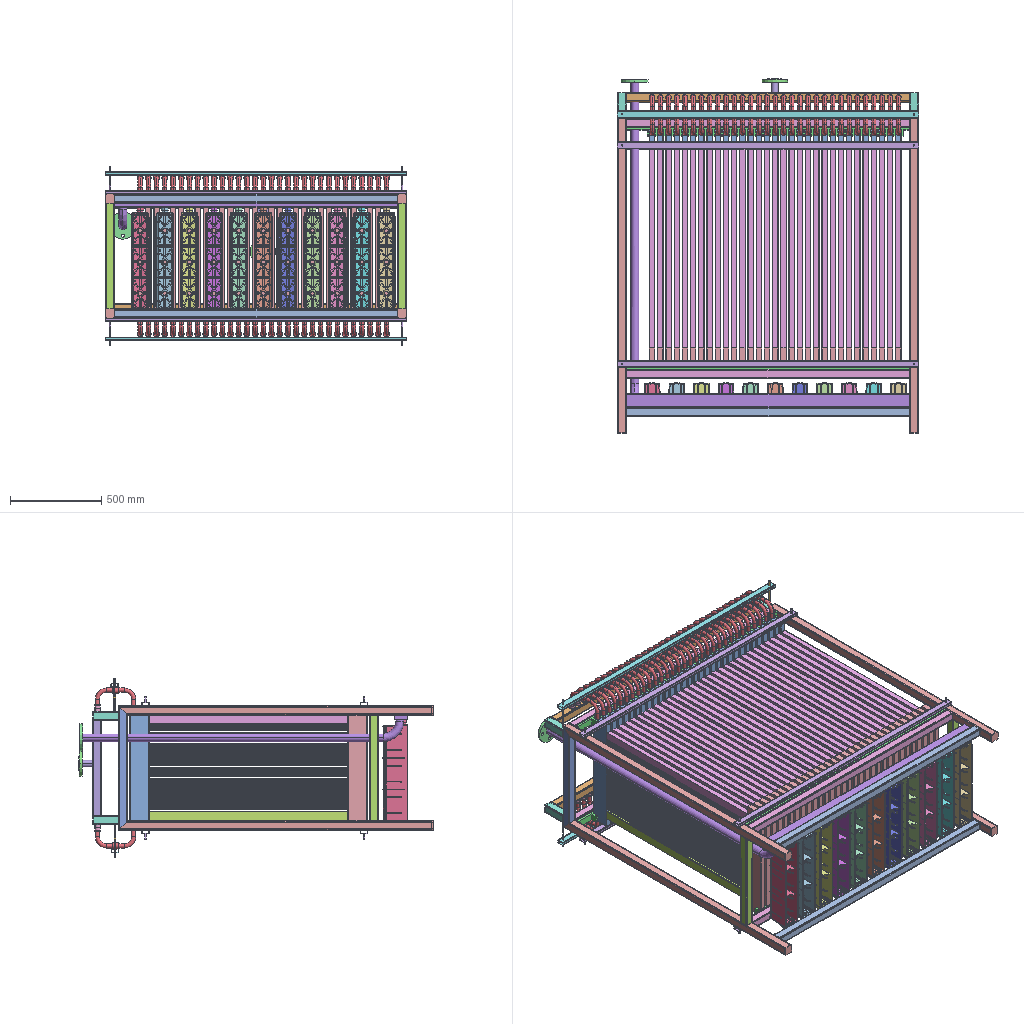Assembly | SolidWorks | 19 different items | 194 placed | box 1650 x 1942 x 981 mm
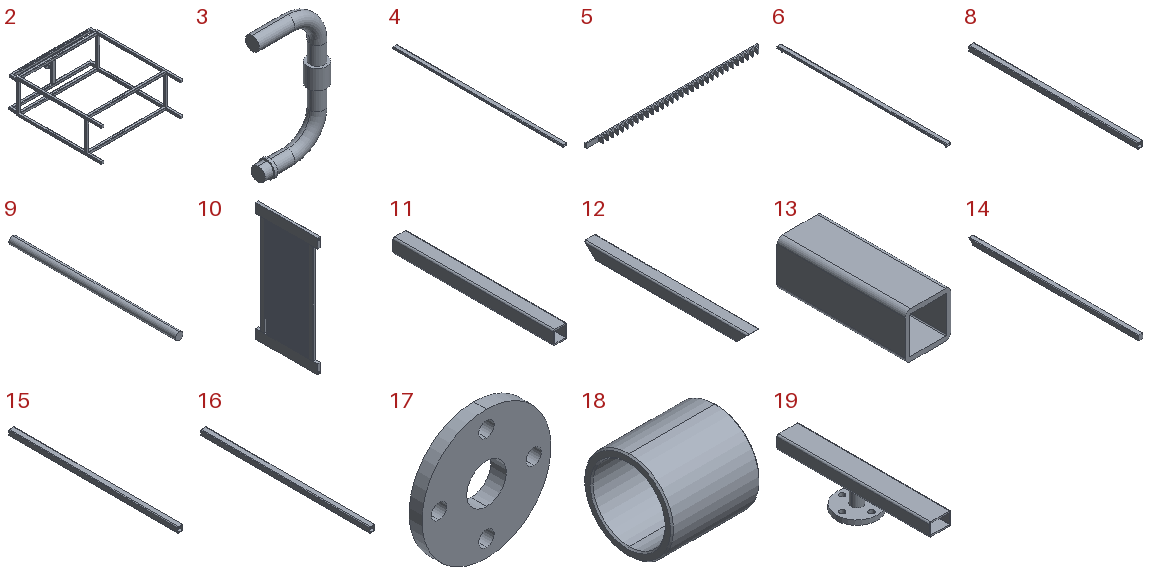Parts list (item | name | quantity | parent item | size | volume | features):
1 | (subassembly) | x1 | - | - | - | features AEMSimFeature 1
2 | (subassembly) | x1 | - | 1650 x 1942 x 680 mm | 17460157 mm3 | features AEMSimFeature 1
3 | - | x62 | - | 127 x 33 x 224.5 mm | 179947 mm3 | features ICE 2, Sweep 1
4 | - | x2 | - | 40 x 1650 x 20 mm | 352604 mm3 | features Extrusion 1
5 | - | x4 | - | 1550 x 48 x 40 mm | 1254000 mm3 | features ICE 8, MoveFace 2, Extrusion 1
6 | - | x4 | - | 40 x 1650 x 50 mm | 355619 mm3 | features Extrusion 1, ICE 1
7 | - | x1 | in 1 | - | - | features ICE 2, BaseBody 1, Fillet 1, MoveCopyBody 1, Sweep 1
8 | - | x2 | - | 50 x 1550 x 50 mm | 1348431 mm3 | features Extrusion 1
9 | - | x4 | - | 8 x 180 x 8 mm | 9048 mm3 | features Extrusion 1
10 | - | x31 | - | 30 x 680 x 1300 mm | 7397272 mm3 | features Fillet 4, ICE 3, Extrusion 1
11 | - | x2 | in 2 | 50 x 580 x 50 mm | 504574 mm3 | features Extrusion 1
12 | - | x2 | in 2 | 50 x 680 x 50 mm | 548072 mm3 | features Extrusion 1, ICE 1
13 | - | x4 | in 2 | 50 x 140 x 50 mm | 129790 mm3 | features Extrusion 1, ICE 1
14 | - | x4 | in 2 | 50 x 1725 x 50 mm | 1494916 mm3 | features ICE 4, Extrusion 1
15 | - | x4 | in 2 | 50 x 1550 x 50 mm | 1348431 mm3 | features Extrusion 1
16 | - | x2 | in 2 | 50 x 1550 x 50 mm | 1299737 mm3 | features ICE 4, Extrusion 1
17 | - | x1 | - | 150 x 18 x 150 mm | 236913 mm3 | features Extrusion 1, ICE 1
18 | - | x62 | - | 30 x 30 x 30 mm | 7020 mm3 | features Revolution 1
19 | - | x1 | in 2 | 140 x 521 x 122 mm | 862843 mm3 | features ICE 4, Extrusion 1
Mates (type | each side: item.copy, entity, surface, feature):
In the top assembly
Coincident | 14.1 face plane Boss-Extrude 1 | assembly face | 2 times
DistanceDim | 14.1 face | assembly face
Coincident | 15.1 face plane Boss-Extrude 1 | 5.1 face plane Boss-Extrude 1 | 2 times
Coincident | 15.2 face plane Boss-Extrude 1 | 5.2 face plane Boss-Extrude 1 | 2 times
Coincident | 5.1 face plane Cut-Extrude 1 | 10.1 face plane Boss-Extrude 1
Coincident | 5.1 face plane Boss-Extrude 1 | 10.1 face plane Boss-Extrude 1
Coincident | 13.1 face plane Boss-Extrude 1 | 9.1 face plane Boss-Extrude 1
DistanceDim | 9.1 face cylinder Boss-Extrude 1 | 12.1 face plane Boss-Extrude 1
DistanceDim | 9.2 face cylinder Boss-Extrude 1 | 12.2 face plane Boss-Extrude 1
DistanceDim | 9.2 face cylinder Boss-Extrude 1 | 13.2 face plane Boss-Extrude 1
Coincident | 13.3 face plane Boss-Extrude 1 | 9.3 face plane Boss-Extrude 1
Concentric | 9.2 face cylinder Boss-Extrude 1 | 9.4 face cylinder Boss-Extrude 1
Coincident | 14.2 face plane Boss-Extrude 1 | 4.1 face plane Boss-Extrude 1
DistanceDim | 9.3 face cylinder Boss-Extrude 1 | 12.1 face plane Boss-Extrude 1
Coincident | 14.2 face plane Boss-Extrude 1 | 6.1 face plane Boss-Extrude 1 | 2 times
Coincident | 14.2 face plane Boss-Extrude 1 | 6.2 face plane Boss-Extrude 1 | 2 times
Coincident | 14.1 face plane Boss-Extrude 1 | 6.3 face plane Boss-Extrude 1 | 2 times
Coincident | 10.1 face plane Boss-Extrude 1 | 6.3 face plane Boss-Extrude 1
Coincident | 14.1 face plane Boss-Extrude 1 | 6.4 face plane Boss-Extrude 1 | 2 times
DistanceDim | 9.3 face cylinder Boss-Extrude 1 | 13.3 face plane Boss-Extrude 1
DistanceDim | 13.1 face plane Boss-Extrude 1 | 9.1 face cylinder Boss-Extrude 1
Coincident | 14.1 face plane Boss-Extrude 1 | 8.1 face plane Boss-Extrude 1 | 2 times
Coincident | 14.2 face plane Boss-Extrude 1 | 8.2 face plane Boss-Extrude 1 | 2 times
Coincident | 14.1 face plane Boss-Extrude 1 | 5.1 face plane Boss-Extrude 2
Coincident | 14.3 face plane Boss-Extrude 1 | 5.2 face plane Boss-Extrude 2
DistanceDim | 10.1 face plane Boss-Extrude 1 | 5.1 face plane Boss-Extrude 4
Concentric | 16.1 face cylinder Cut-Extrude 2 | 18.1 face cylinder Revolve 1
Coincident | 16.1 face plane Boss-Extrude 1 | 18.1 face plane Revolve 1
Coincident | 7.1 face plane Boss-Extrude 1 | 8.1 face plane Boss-Extrude 1
Coincident | 14.4 face plane Boss-Extrude 1 | 7.1 face plane Boss-Extrude 1
Concentric | 7.1 face cylinder Sweep 1 | 17.1 face cylinder Boss-Extrude 1
Coincident | 7.1 face plane Sweep 1 | 17.1 face plane Boss-Extrude 2
Coincident | 13.2 face plane Boss-Extrude 1 | 9.2 face plane Boss-Extrude 1
Coincident | 13.4 face plane Boss-Extrude 1 | 9.4 edge
Coincident | 15.3 face plane Boss-Extrude 1 | 5.3 face plane Boss-Extrude 1
Coincident | 14.3 face plane Boss-Extrude 1 | 5.3 face plane Boss-Extrude 2
Coincident | 5.3 face plane Boss-Extrude 1 | 5.2 face plane Boss-Extrude 1
Coincident | 15.4 face plane Boss-Extrude 1 | 5.4 face plane Boss-Extrude 1
Coincident | 5.1 face plane Boss-Extrude 1 | 5.4 face plane Boss-Extrude 1
Coincident | 14.1 face plane Boss-Extrude 1 | 5.4 face plane Boss-Extrude 2
Concentric | 16.2 face cylinder Cut-Extrude 2 | 18.2 face cylinder Revolve 1
Coincident | 16.2 face plane Boss-Extrude 1 | 18.2 face plane Revolve 1
Concentric | 18.2 face cylinder Revolve 1 | 3.1 face cylinder Sweep 1
Coincident | 18.2 face plane Revolve 1 | 3.1 face plane Boss-Extrude 1
Concentric | 18.1 face cylinder Revolve 1 | 3.2 face cylinder Sweep 1
Coincident | 18.1 face plane Revolve 1 | 3.2 face plane Boss-Extrude 1
Concentric | 3.1 face cylinder Sweep 1 | 3.2 face cylinder Sweep 1
In subassembly 2
Coincident | 14.5 face plane Boss-Extrude 1 | 12.3 face plane Boss-Extrude 1
Coincident | 14.5 face plane Cut-Extrude 1 | 12.3 face plane Cut-Extrude 1
Coincident | 14.5 edge | 12.3 face plane Boss-Extrude 1
Coincident | 12.3 face plane Boss-Extrude 1 | 14.6 face plane Boss-Extrude 1
Coincident | 12.3 face plane Cut-Extrude 1 | 14.6 face plane Cut-Extrude 1
Coincident | 12.3 face plane Boss-Extrude 1 | 14.6 edge
Coincident | 14.5 face plane Boss-Extrude 1 | 11.1 face plane Boss-Extrude 1 | 2 times
Coincident | 14.6 face plane Boss-Extrude 1 | 15.5 face plane Boss-Extrude 1 | 2 times
Coincident | 12.3 face plane Boss-Extrude 1 | 15.5 face plane Boss-Extrude 1
Coincident | 12.3 face plane Boss-Extrude 1 | 15.6 face plane Boss-Extrude 1 | 2 times
Coincident | 14.5 face plane Boss-Extrude 1 | 15.6 face plane Boss-Extrude 1
Coincident | 14.6 face plane Boss-Extrude 1 | 15.7 face plane Boss-Extrude 1 | 2 times
Coincident | 11.1 face plane Boss-Extrude 1 | 15.7 face plane Boss-Extrude 1
Coincident | 11.1 face plane Boss-Extrude 1 | 15.8 face plane Boss-Extrude 1
Coincident | 14.5 face plane Boss-Extrude 1 | 15.8 face plane Boss-Extrude 1 | 2 times
Coincident | 12.4 face plane Boss-Extrude 1 | 14.7 face plane Boss-Extrude 1
Coincident | 12.4 face plane Cut-Extrude 1 | 14.7 face plane Cut-Extrude 1
Coincident | 12.4 face plane Boss-Extrude 1 | 14.8 face plane Boss-Extrude 1
Coincident | 12.4 face plane Cut-Extrude 1 | 14.8 face plane Cut-Extrude 1
Coincident | 12.4 face plane Boss-Extrude 1 | 14.8 edge
Coincident | 12.4 face plane Boss-Extrude 1 | 14.7 edge
Coincident | 15.6 face plane Boss-Extrude 1 | 12.4 face plane Boss-Extrude 1
Coincident | 15.5 face plane Boss-Extrude 1 | 14.7 face plane Boss-Extrude 1
Coincident | 15.5 face plane Boss-Extrude 1 | 12.4 face plane Boss-Extrude 1
Coincident | 11.1 face plane Boss-Extrude 1 | 11.2 face plane Boss-Extrude 1
Coincident | 14.7 face plane Boss-Extrude 1 | 11.2 face plane Boss-Extrude 1 | 2 times
Coincident | 12.3 face plane Boss-Extrude 1 | 13.5 face plane Boss-Extrude 1 | 2 times
Coincident | 12.4 face plane Boss-Extrude 1 | 13.6 face plane Boss-Extrude 1
Coincident | 13.5 face plane Boss-Extrude 1 | 13.6 face plane Boss-Extrude 1
Coincident | 13.7 face plane Boss-Extrude 1 | 16.3 face plane Boss-Extrude 1 | 3 times
Coincident | 16.3 face plane Boss-Extrude 1 | 19.1 face plane Boss-Extrude 1 | 2 times
Coincident | 12.3 face plane Boss-Extrude 1 | 13.8 face plane Boss-Extrude 1 | 2 times
Coincident | 13.8 face plane Boss-Extrude 1 | 16.3 face plane Boss-Extrude 1 | 3 times
DistanceDim | 13.5 face plane Boss-Extrude 1 | 14.6 face plane Boss-Extrude 1
DistanceDim | 19.1 face plane Boss-Extrude 1 | 13.7 face plane Boss-Extrude 1
Coincident | 13.6 face plane Boss-Extrude 1 | 16.4 face plane Boss-Extrude 1 | 3 times